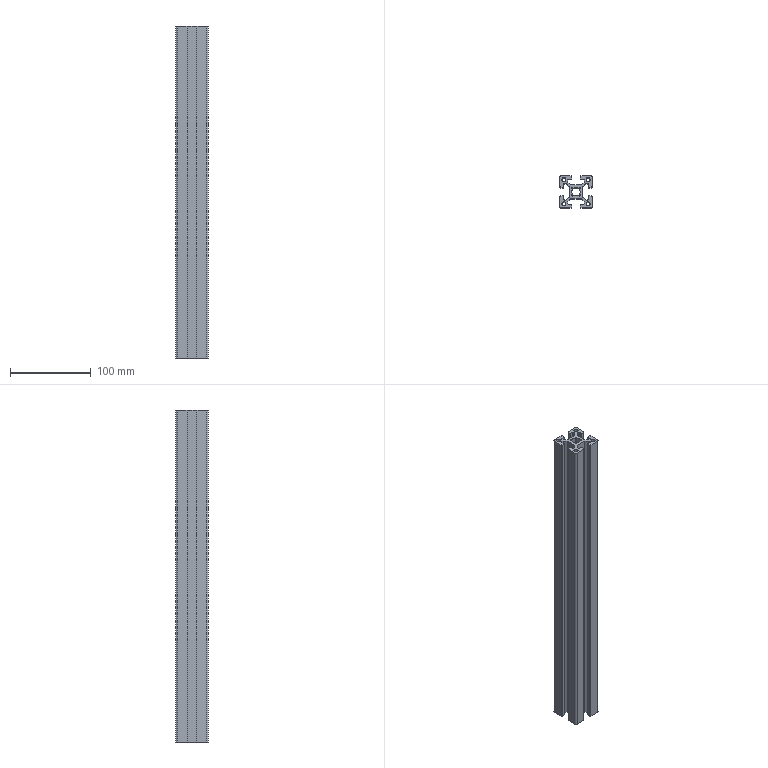Part | SolidWorks | features Extrusion 1 | 1 solid | 125 faces | box 40 x 40 x 410 mm | volume 287601 mm3 | plane 74 | cylinder 51 | commonest cylinder face diameters 2 x24 1.5 x10 5 x8 10.2 x5 4 x4